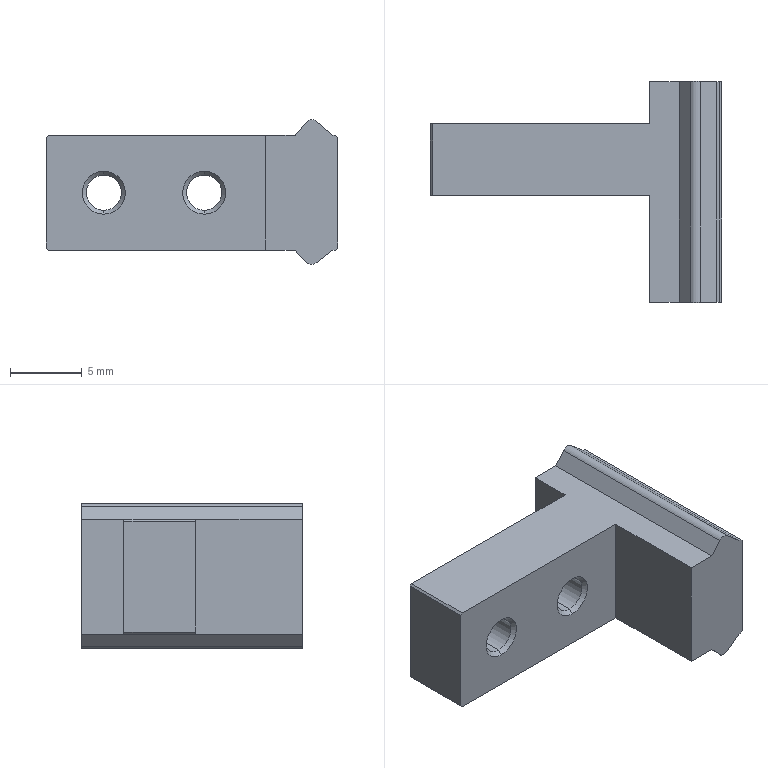Part | SolidWorks | features BaseBody 1 | 1 solid | 35 faces | box 20.3 x 15.4 x 10.1 mm | volume 1229 mm3 | plane 20 | cone 8 | cylinder 7 | commonest cylinder face diameters 2.459 x4 1 x3
STEP:
#1=CARTESIAN_POINT('',(-55.8,12.19,-1.229));
#2=VERTEX_POINT('',#1);
#3=CARTESIAN_POINT('',(-55.8,12.19,1.229));
#4=VERTEX_POINT('',#3);
#5=CARTESIAN_POINT('',(-55.8,12.19,0.));
#6=DIRECTION('',(0.,1.,0.));
#7=DIRECTION('',(0.,0.,1.));
#8=AXIS2_PLACEMENT_3D('',#5,#6,#7);
#9=CIRCLE('',#8,1.229);
#10=EDGE_CURVE('',#2,#4,#9,.T.);
#11=ORIENTED_EDGE('',*,*,#10,.F.);
#12=CARTESIAN_POINT('',(-55.8,12.46,-1.5));
#13=VERTEX_POINT('',#12);
#14=CARTESIAN_POINT('',(-55.8,12.19,-1.229));
#15=DIRECTION('',(0.,0.7071,-0.7071));
#16=VECTOR('',#15,1000.);
#17=LINE('',#14,#16);
#18=EDGE_CURVE('',#2,#13,#17,.T.);
#19=ORIENTED_EDGE('',*,*,#18,.T.);
#20=CARTESIAN_POINT('',(-55.8,12.46,1.5));
#21=VERTEX_POINT('',#20);
#22=CARTESIAN_POINT('',(-55.8,12.46,0.));
#23=DIRECTION('',(0.,1.,0.));
#24=DIRECTION('',(0.,0.,1.));
#25=AXIS2_PLACEMENT_3D('',#22,#23,#24);
#26=CIRCLE('',#25,1.5);
#27=EDGE_CURVE('',#13,#21,#26,.T.);
#28=ORIENTED_EDGE('',*,*,#27,.T.);
#29=CARTESIAN_POINT('',(-55.8,12.19,1.229));
#30=DIRECTION('',(0.,0.7071,0.7071));
#31=VECTOR('',#30,1000.);
#32=LINE('',#29,#31);
#33=EDGE_CURVE('',#4,#21,#32,.T.);
#34=ORIENTED_EDGE('',*,*,#33,.F.);
#35=EDGE_LOOP('',(#11,#19,#28,#34));
#36=FACE_OUTER_BOUND('',#35,.T.);
#37=CARTESIAN_POINT('',(-55.8,12.19,0.));
#38=DIRECTION('',(0.,1.,0.));
#39=DIRECTION('',(0.,0.,1.));
#40=AXIS2_PLACEMENT_3D('',#37,#38,#39);
#41=CONICAL_SURFACE('',#40,1.229,0.7854);
#42=ADVANCED_FACE('',(#36),#41,.F.);
#43=CARTESIAN_POINT('',(-55.8,7.721,-1.229));
#44=VERTEX_POINT('',#43);
#45=CARTESIAN_POINT('',(-55.8,7.721,1.229));
#46=VERTEX_POINT('',#45);
#47=CARTESIAN_POINT('',(-55.8,7.721,0.));
#48=DIRECTION('',(0.,1.,0.));
#49=DIRECTION('',(0.,0.,1.));
#50=AXIS2_PLACEMENT_3D('',#47,#48,#49);
#51=CIRCLE('',#50,1.229);
#52=EDGE_CURVE('',#44,#46,#51,.T.);
#53=ORIENTED_EDGE('',*,*,#52,.F.);
#54=CARTESIAN_POINT('',(-55.8,12.46,-1.229));
#55=DIRECTION('',(0.,1.,0.));
#56=VECTOR('',#55,1000.);
#57=LINE('',#54,#56);
#58=EDGE_CURVE('',#44,#2,#57,.T.);
#59=ORIENTED_EDGE('',*,*,#58,.T.);
#60=ORIENTED_EDGE('',*,*,#10,.T.);
#61=CARTESIAN_POINT('',(-55.8,12.46,1.229));
#62=DIRECTION('',(0.,1.,0.));
#63=VECTOR('',#62,1000.);
#64=LINE('',#61,#63);
#65=EDGE_CURVE('',#46,#4,#64,.T.);
#66=ORIENTED_EDGE('',*,*,#65,.F.);
#67=EDGE_LOOP('',(#53,#59,#60,#66));
#68=FACE_OUTER_BOUND('',#67,.T.);
#69=CARTESIAN_POINT('',(-55.8,12.46,0.));
#70=DIRECTION('',(0.,1.,0.));
#71=DIRECTION('',(0.,0.,1.));
#72=AXIS2_PLACEMENT_3D('',#69,#70,#71);
#73=CYLINDRICAL_SURFACE('',#72,1.229);
#74=ADVANCED_FACE('',(#68),#73,.F.);
#75=ORIENTED_EDGE('',*,*,#52,.T.);
#76=CARTESIAN_POINT('',(-55.8,7.45,1.5));
#77=VERTEX_POINT('',#76);
#78=CARTESIAN_POINT('',(-55.8,7.45,1.5));
#79=DIRECTION('',(0.,-0.7071,0.7071));
#80=VECTOR('',#79,1000.);
#81=LINE('',#78,#80);
#82=EDGE_CURVE('',#46,#77,#81,.T.);
#83=ORIENTED_EDGE('',*,*,#82,.T.);
#84=CARTESIAN_POINT('',(-55.8,7.45,-1.5));
#85=VERTEX_POINT('',#84);
#86=CARTESIAN_POINT('',(-55.8,7.45,0.));
#87=DIRECTION('',(0.,1.,0.));
#88=DIRECTION('',(0.,0.,1.));
#89=AXIS2_PLACEMENT_3D('',#86,#87,#88);
#90=CIRCLE('',#89,1.5);
#91=EDGE_CURVE('',#85,#77,#90,.T.);
#92=ORIENTED_EDGE('',*,*,#91,.F.);
#93=CARTESIAN_POINT('',(-55.8,7.45,-1.5));
#94=DIRECTION('',(0.,-0.7071,-0.7071));
#95=VECTOR('',#94,1000.);
#96=LINE('',#93,#95);
#97=EDGE_CURVE('',#44,#85,#96,.T.);
#98=ORIENTED_EDGE('',*,*,#97,.F.);
#99=EDGE_LOOP('',(#75,#83,#92,#98));
#100=FACE_OUTER_BOUND('',#99,.T.);
#101=CARTESIAN_POINT('',(-55.8,7.45,0.));
#102=DIRECTION('',(0.,-1.,0.));
#103=DIRECTION('',(0.,0.,-1.));
#104=AXIS2_PLACEMENT_3D('',#101,#102,#103);
#105=CONICAL_SURFACE('',#104,1.5,0.7854);
#106=ADVANCED_FACE('',(#100),#105,.F.);
#107=CARTESIAN_POINT('',(-62.8,12.19,-1.229));
#108=VERTEX_POINT('',#107);
#109=CARTESIAN_POINT('',(-62.8,12.19,1.229));
#110=VERTEX_POINT('',#109);
#111=CARTESIAN_POINT('',(-62.8,12.19,0.));
#112=DIRECTION('',(0.,1.,0.));
#113=DIRECTION('',(0.,0.,1.));
#114=AXIS2_PLACEMENT_3D('',#111,#112,#113);
#115=CIRCLE('',#114,1.229);
#116=EDGE_CURVE('',#108,#110,#115,.T.);
#117=ORIENTED_EDGE('',*,*,#116,.F.);
#118=CARTESIAN_POINT('',(-62.8,12.46,-1.5));
#119=VERTEX_POINT('',#118);
#120=CARTESIAN_POINT('',(-62.8,12.19,-1.229));
#121=DIRECTION('',(0.,0.7071,-0.7071));
#122=VECTOR('',#121,1000.);
#123=LINE('',#120,#122);
#124=EDGE_CURVE('',#108,#119,#123,.T.);
#125=ORIENTED_EDGE('',*,*,#124,.T.);
#126=CARTESIAN_POINT('',(-62.8,12.46,1.5));
#127=VERTEX_POINT('',#126);
#128=CARTESIAN_POINT('',(-62.8,12.46,0.));
#129=DIRECTION('',(0.,1.,0.));
#130=DIRECTION('',(0.,0.,1.));
#131=AXIS2_PLACEMENT_3D('',#128,#129,#130);
#132=CIRCLE('',#131,1.5);
#133=EDGE_CURVE('',#119,#127,#132,.T.);
#134=ORIENTED_EDGE('',*,*,#133,.T.);
#135=CARTESIAN_POINT('',(-62.8,12.19,1.229));
#136=DIRECTION('',(0.,0.7071,0.7071));
#137=VECTOR('',#136,1000.);
#138=LINE('',#135,#137);
#139=EDGE_CURVE('',#110,#127,#138,.T.);
#140=ORIENTED_EDGE('',*,*,#139,.F.);
#141=EDGE_LOOP('',(#117,#125,#134,#140));
#142=FACE_OUTER_BOUND('',#141,.T.);
#143=CARTESIAN_POINT('',(-62.8,12.19,0.));
#144=DIRECTION('',(0.,1.,0.));
#145=DIRECTION('',(0.,0.,1.));
#146=AXIS2_PLACEMENT_3D('',#143,#144,#145);
#147=CONICAL_SURFACE('',#146,1.229,0.7854);
#148=ADVANCED_FACE('',(#142),#147,.F.);
#149=CARTESIAN_POINT('',(-62.8,7.721,-1.229));
#150=VERTEX_POINT('',#149);
#151=CARTESIAN_POINT('',(-62.8,7.721,1.229));
#152=VERTEX_POINT('',#151);
#153=CARTESIAN_POINT('',(-62.8,7.721,0.));
#154=DIRECTION('',(0.,1.,0.));
#155=DIRECTION('',(0.,0.,1.));
#156=AXIS2_PLACEMENT_3D('',#153,#154,#155);
#157=CIRCLE('',#156,1.229);
#158=EDGE_CURVE('',#150,#152,#157,.T.);
#159=ORIENTED_EDGE('',*,*,#158,.F.);
#160=CARTESIAN_POINT('',(-62.8,12.46,-1.229));
#161=DIRECTION('',(0.,1.,0.));
#162=VECTOR('',#161,1000.);
#163=LINE('',#160,#162);
#164=EDGE_CURVE('',#150,#108,#163,.T.);
#165=ORIENTED_EDGE('',*,*,#164,.T.);
#166=ORIENTED_EDGE('',*,*,#116,.T.);
#167=CARTESIAN_POINT('',(-62.8,12.46,1.229));
#168=DIRECTION('',(0.,1.,0.));
#169=VECTOR('',#168,1000.);
#170=LINE('',#167,#169);
#171=EDGE_CURVE('',#152,#110,#170,.T.);
#172=ORIENTED_EDGE('',*,*,#171,.F.);
#173=EDGE_LOOP('',(#159,#165,#166,#172));
#174=FACE_OUTER_BOUND('',#173,.T.);
#175=CARTESIAN_POINT('',(-62.8,12.46,0.));
#176=DIRECTION('',(0.,1.,0.));
#177=DIRECTION('',(0.,0.,1.));
#178=AXIS2_PLACEMENT_3D('',#175,#176,#177);
#179=CYLINDRICAL_SURFACE('',#178,1.229);
#180=ADVANCED_FACE('',(#174),#179,.F.);
#181=ORIENTED_EDGE('',*,*,#158,.T.);
#182=CARTESIAN_POINT('',(-62.8,7.45,1.5));
#183=VERTEX_POINT('',#182);
#184=CARTESIAN_POINT('',(-62.8,7.45,1.5));
#185=DIRECTION('',(0.,-0.7071,0.7071));
#186=VECTOR('',#185,1000.);
#187=LINE('',#184,#186);
#188=EDGE_CURVE('',#152,#183,#187,.T.);
#189=ORIENTED_EDGE('',*,*,#188,.T.);
#190=CARTESIAN_POINT('',(-62.8,7.45,-1.5));
#191=VERTEX_POINT('',#190);
#192=CARTESIAN_POINT('',(-62.8,7.45,0.));
#193=DIRECTION('',(0.,1.,0.));
#194=DIRECTION('',(0.,0.,1.));
#195=AXIS2_PLACEMENT_3D('',#192,#193,#194);
#196=CIRCLE('',#195,1.5);
#197=EDGE_CURVE('',#191,#183,#196,.T.);
#198=ORIENTED_EDGE('',*,*,#197,.F.);
#199=CARTESIAN_POINT('',(-62.8,7.45,-1.5));
#200=DIRECTION('',(0.,-0.7071,-0.7071));
#201=VECTOR('',#200,1000.);
#202=LINE('',#199,#201);
#203=EDGE_CURVE('',#150,#191,#202,.T.);
#204=ORIENTED_EDGE('',*,*,#203,.F.);
#205=EDGE_LOOP('',(#181,#189,#198,#204));
#206=FACE_OUTER_BOUND('',#205,.T.);
#207=CARTESIAN_POINT('',(-62.8,7.45,0.));
#208=DIRECTION('',(0.,-1.,0.));
#209=DIRECTION('',(0.,0.,-1.));
#210=AXIS2_PLACEMENT_3D('',#207,#208,#209);
#211=CONICAL_SURFACE('',#210,1.5,0.7854);
#212=ADVANCED_FACE('',(#206),#211,.F.);
#213=CARTESIAN_POINT('',(-48.3,15.41,-5.));
#214=VERTEX_POINT('',#213);
#215=CARTESIAN_POINT('',(-48.663,15.41,-4.843));
#216=VERTEX_POINT('',#215);
#217=CARTESIAN_POINT('',(-48.3,15.41,-4.5));
#218=DIRECTION('',(0.,1.,0.));
#219=DIRECTION('',(0.6065,0.,-0.7951));
#220=AXIS2_PLACEMENT_3D('',#217,#218,#219);
#221=CIRCLE('',#220,0.5);
#222=EDGE_CURVE('',#214,#216,#221,.T.);
#223=ORIENTED_EDGE('',*,*,#222,.F.);
#224=CARTESIAN_POINT('',(-48.3,0.01,-5.));
#225=VERTEX_POINT('',#224);
#226=CARTESIAN_POINT('',(-48.3,15.41,-5.));
#227=DIRECTION('',(0.,-1.,0.));
#228=VECTOR('',#227,1000.);
#229=LINE('',#226,#228);
#230=EDGE_CURVE('',#214,#225,#229,.T.);
#231=ORIENTED_EDGE('',*,*,#230,.T.);
#232=CARTESIAN_POINT('',(-48.663,0.01,-4.843));
#233=VERTEX_POINT('',#232);
#234=CARTESIAN_POINT('',(-48.3,0.01,-4.5));
#235=DIRECTION('',(0.,1.,0.));
#236=DIRECTION('',(0.6065,0.,-0.7951));
#237=AXIS2_PLACEMENT_3D('',#234,#235,#236);
#238=CIRCLE('',#237,0.5);
#239=EDGE_CURVE('',#225,#233,#238,.T.);
#240=ORIENTED_EDGE('',*,*,#239,.T.);
#241=CARTESIAN_POINT('',(-48.663,15.41,-4.843));
#242=DIRECTION('',(0.,-1.,0.));
#243=VECTOR('',#242,1000.);
#244=LINE('',#241,#243);
#245=EDGE_CURVE('',#216,#233,#244,.T.);
#246=ORIENTED_EDGE('',*,*,#245,.F.);
#247=EDGE_LOOP('',(#223,#231,#240,#246));
#248=FACE_OUTER_BOUND('',#247,.T.);
#249=CARTESIAN_POINT('',(-48.3,15.41,-4.5));
#250=DIRECTION('',(0.,-1.,0.));
#251=DIRECTION('',(0.,0.,-1.));
#252=AXIS2_PLACEMENT_3D('',#249,#250,#251);
#253=CYLINDRICAL_SURFACE('',#252,0.5);
#254=ADVANCED_FACE('',(#248),#253,.T.);
#255=CARTESIAN_POINT('',(-51.5,12.46,4.));
#256=VERTEX_POINT('',#255);
#257=CARTESIAN_POINT('',(-51.5,12.46,-4.));
#258=VERTEX_POINT('',#257);
#259=CARTESIAN_POINT('',(-51.5,12.46,4.));
#260=DIRECTION('',(0.,0.,-1.));
#261=VECTOR('',#260,1000.);
#262=LINE('',#259,#261);
#263=EDGE_CURVE('',#256,#258,#262,.T.);
#264=ORIENTED_EDGE('',*,*,#263,.F.);
#265=CARTESIAN_POINT('',(-51.5,15.41,4.));
#266=VERTEX_POINT('',#265);
#267=CARTESIAN_POINT('',(-51.5,15.41,4.));
#268=DIRECTION('',(0.,-1.,0.));
#269=VECTOR('',#268,1000.);
#270=LINE('',#267,#269);
#271=EDGE_CURVE('',#266,#256,#270,.T.);
#272=ORIENTED_EDGE('',*,*,#271,.F.);
#273=CARTESIAN_POINT('',(-51.5,15.41,-4.));
#274=VERTEX_POINT('',#273);
#275=CARTESIAN_POINT('',(-51.5,15.41,-4.));
#276=DIRECTION('',(0.,0.,1.));
#277=VECTOR('',#276,1000.);
#278=LINE('',#275,#277);
#279=EDGE_CURVE('',#274,#266,#278,.T.);
#280=ORIENTED_EDGE('',*,*,#279,.F.);
#281=CARTESIAN_POINT('',(-51.5,15.41,-4.));
#282=DIRECTION('',(0.,-1.,0.));
#283=VECTOR('',#282,1000.);
#284=LINE('',#281,#283);
#285=EDGE_CURVE('',#274,#258,#284,.T.);
#286=ORIENTED_EDGE('',*,*,#285,.T.);
#287=EDGE_LOOP('',(#264,#272,#280,#286));
#288=FACE_OUTER_BOUND('',#287,.T.);
#289=CARTESIAN_POINT('',(-51.5,15.41,-4.));
#290=DIRECTION('',(1.,0.,0.));
#291=DIRECTION('',(0.,0.,-1.));
#292=AXIS2_PLACEMENT_3D('',#289,#290,#291);
#293=PLANE('',#292);
#294=ADVANCED_FACE('',(#288),#293,.F.);
#295=CARTESIAN_POINT('',(-51.5,7.45,4.));
#296=VERTEX_POINT('',#295);
#297=CARTESIAN_POINT('',(-51.5,0.01,4.));
#298=VERTEX_POINT('',#297);
#299=CARTESIAN_POINT('',(-51.5,7.45,4.));
#300=DIRECTION('',(0.,-1.,0.));
#301=VECTOR('',#300,1000.);
#302=LINE('',#299,#301);
#303=EDGE_CURVE('',#296,#298,#302,.T.);
#304=ORIENTED_EDGE('',*,*,#303,.F.);
#305=CARTESIAN_POINT('',(-51.5,7.45,-4.));
#306=VERTEX_POINT('',#305);
#307=CARTESIAN_POINT('',(-51.5,7.45,4.));
#308=DIRECTION('',(0.,0.,-1.));
#309=VECTOR('',#308,1000.);
#310=LINE('',#307,#309);
#311=EDGE_CURVE('',#296,#306,#310,.T.);
#312=ORIENTED_EDGE('',*,*,#311,.T.);
#313=CARTESIAN_POINT('',(-51.5,0.01,-4.));
#314=VERTEX_POINT('',#313);
#315=CARTESIAN_POINT('',(-51.5,7.45,-4.));
#316=DIRECTION('',(0.,-1.,0.));
#317=VECTOR('',#316,1000.);
#318=LINE('',#315,#317);
#319=EDGE_CURVE('',#306,#314,#318,.T.);
#320=ORIENTED_EDGE('',*,*,#319,.T.);
#321=CARTESIAN_POINT('',(-51.5,0.01,-4.));
#322=DIRECTION('',(0.,0.,1.));
#323=VECTOR('',#322,1000.);
#324=LINE('',#321,#323);
#325=EDGE_CURVE('',#314,#298,#324,.T.);
#326=ORIENTED_EDGE('',*,*,#325,.T.);
#327=EDGE_LOOP('',(#304,#312,#320,#326));
#328=FACE_OUTER_BOUND('',#327,.T.);
#329=CARTESIAN_POINT('',(-51.5,15.41,-4.));
#330=DIRECTION('',(1.,0.,0.));
#331=DIRECTION('',(0.,0.,-1.));
#332=AXIS2_PLACEMENT_3D('',#329,#330,#331);
#333=PLANE('',#332);
#334=ADVANCED_FACE('',(#328),#333,.F.);
#335=CARTESIAN_POINT('',(-49.46,0.01,4.));
#336=VERTEX_POINT('',#335);
#337=CARTESIAN_POINT('',(-51.5,0.01,4.));
#338=DIRECTION('',(1.,0.,0.));
#339=VECTOR('',#338,1000.);
#340=LINE('',#337,#339);
#341=EDGE_CURVE('',#298,#336,#340,.T.);
#342=ORIENTED_EDGE('',*,*,#341,.T.);
#343=CARTESIAN_POINT('',(-49.46,15.41,4.));
#344=VERTEX_POINT('',#343);
#345=CARTESIAN_POINT('',(-49.46,15.41,4.));
#346=DIRECTION('',(0.,-1.,0.));
#347=VECTOR('',#346,1000.);
#348=LINE('',#345,#347);
#349=EDGE_CURVE('',#344,#336,#348,.T.);
#350=ORIENTED_EDGE('',*,*,#349,.F.);
#351=CARTESIAN_POINT('',(-51.5,15.41,4.));
#352=DIRECTION('',(1.,0.,0.));
#353=VECTOR('',#352,1000.);
#354=LINE('',#351,#353);
#355=EDGE_CURVE('',#266,#344,#354,.T.);
#356=ORIENTED_EDGE('',*,*,#355,.F.);
#357=ORIENTED_EDGE('',*,*,#271,.T.);
#358=CARTESIAN_POINT('',(-66.659,12.46,4.));
#359=VERTEX_POINT('',#358);
#360=CARTESIAN_POINT('',(-66.659,12.46,4.));
#361=DIRECTION('',(1.,0.,0.));
#362=VECTOR('',#361,1000.);
#363=LINE('',#360,#362);
#364=EDGE_CURVE('',#359,#256,#363,.T.);
#365=ORIENTED_EDGE('',*,*,#364,.F.);
#366=CARTESIAN_POINT('',(-66.659,7.45,4.));
#367=VERTEX_POINT('',#366);
#368=CARTESIAN_POINT('',(-66.659,12.46,4.));
#369=DIRECTION('',(0.,-1.,0.));
#370=VECTOR('',#369,1000.);
#371=LINE('',#368,#370);
#372=EDGE_CURVE('',#359,#367,#371,.T.);
#373=ORIENTED_EDGE('',*,*,#372,.T.);
#374=CARTESIAN_POINT('',(-66.659,7.45,4.));
#375=DIRECTION('',(1.,0.,0.));
#376=VECTOR('',#375,1000.);
#377=LINE('',#374,#376);
#378=EDGE_CURVE('',#367,#296,#377,.T.);
#379=ORIENTED_EDGE('',*,*,#378,.T.);
#380=ORIENTED_EDGE('',*,*,#303,.T.);
#381=EDGE_LOOP('',(#342,#350,#356,#357,#365,#373,#379,#380));
#382=FACE_OUTER_BOUND('',#381,.T.);
#383=CARTESIAN_POINT('',(-51.5,15.41,4.));
#384=DIRECTION('',(0.,0.,-1.));
#385=DIRECTION('',(-1.,0.,0.));
#386=AXIS2_PLACEMENT_3D('',#383,#384,#385);
#387=PLANE('',#386);
#388=ADVANCED_FACE('',(#382),#387,.F.);
#389=CARTESIAN_POINT('',(-48.682,0.01,4.922));
#390=VERTEX_POINT('',#389);
#391=CARTESIAN_POINT('',(-49.46,0.01,4.));
#392=DIRECTION('',(0.6447,0.,0.7645));
#393=VECTOR('',#392,1000.);
#394=LINE('',#391,#393);
#395=EDGE_CURVE('',#336,#390,#394,.T.);
#396=ORIENTED_EDGE('',*,*,#395,.T.);
#397=CARTESIAN_POINT('',(-48.682,15.41,4.922));
#398=VERTEX_POINT('',#397);
#399=CARTESIAN_POINT('',(-48.682,15.41,4.922));
#400=DIRECTION('',(0.,-1.,0.));
#401=VECTOR('',#400,1000.);
#402=LINE('',#399,#401);
#403=EDGE_CURVE('',#398,#390,#402,.T.);
#404=ORIENTED_EDGE('',*,*,#403,.F.);
#405=CARTESIAN_POINT('',(-49.46,15.41,4.));
#406=DIRECTION('',(0.6447,0.,0.7645));
#407=VECTOR('',#406,1000.);
#408=LINE('',#405,#407);
#409=EDGE_CURVE('',#344,#398,#408,.T.);
#410=ORIENTED_EDGE('',*,*,#409,.F.);
#411=ORIENTED_EDGE('',*,*,#349,.T.);
#412=EDGE_LOOP('',(#396,#404,#410,#411));
#413=FACE_OUTER_BOUND('',#412,.T.);
#414=CARTESIAN_POINT('',(-49.46,15.41,4.));
#415=DIRECTION('',(0.7645,0.,-0.6447));
#416=DIRECTION('',(-0.6447,0.,-0.7645));
#417=AXIS2_PLACEMENT_3D('',#414,#415,#416);
#418=PLANE('',#417);
#419=ADVANCED_FACE('',(#413),#418,.F.);
#420=CARTESIAN_POINT('',(-47.977,0.01,4.981));
#421=VERTEX_POINT('',#420);
#422=CARTESIAN_POINT('',(-48.3,0.01,4.6));
#423=DIRECTION('',(0.,1.,0.));
#424=DIRECTION('',(-0.7645,0.,0.6447));
#425=AXIS2_PLACEMENT_3D('',#422,#423,#424);
#426=CIRCLE('',#425,0.5);
#427=EDGE_CURVE('',#390,#421,#426,.T.);
#428=ORIENTED_EDGE('',*,*,#427,.T.);
#429=CARTESIAN_POINT('',(-47.977,15.41,4.981));
#430=VERTEX_POINT('',#429);
#431=CARTESIAN_POINT('',(-47.977,15.41,4.981));
#432=DIRECTION('',(0.,-1.,0.));
#433=VECTOR('',#432,1000.);
#434=LINE('',#431,#433);
#435=EDGE_CURVE('',#430,#421,#434,.T.);
#436=ORIENTED_EDGE('',*,*,#435,.F.);
#437=CARTESIAN_POINT('',(-48.3,15.41,4.6));
#438=DIRECTION('',(0.,1.,0.));
#439=DIRECTION('',(-0.7645,0.,0.6447));
#440=AXIS2_PLACEMENT_3D('',#437,#438,#439);
#441=CIRCLE('',#440,0.5);
#442=EDGE_CURVE('',#398,#430,#441,.T.);
#443=ORIENTED_EDGE('',*,*,#442,.F.);
#444=ORIENTED_EDGE('',*,*,#403,.T.);
#445=EDGE_LOOP('',(#428,#436,#443,#444));
#446=FACE_OUTER_BOUND('',#445,.T.);
#447=CARTESIAN_POINT('',(-48.3,15.41,4.6));
#448=DIRECTION('',(0.,-1.,0.));
#449=DIRECTION('',(0.,0.,-1.));
#450=AXIS2_PLACEMENT_3D('',#447,#448,#449);
#451=CYLINDRICAL_SURFACE('',#450,0.5);
#452=ADVANCED_FACE('',(#446),#451,.T.);
#453=CARTESIAN_POINT('',(-46.82,0.01,4.));
#454=VERTEX_POINT('',#453);
#455=CARTESIAN_POINT('',(-47.977,0.01,4.981));
#456=DIRECTION('',(0.7625,0.,-0.647));
#457=VECTOR('',#456,1000.);
#458=LINE('',#455,#457);
#459=EDGE_CURVE('',#421,#454,#458,.T.);
#460=ORIENTED_EDGE('',*,*,#459,.T.);
#461=CARTESIAN_POINT('',(-46.82,15.41,4.));
#462=VERTEX_POINT('',#461);
#463=CARTESIAN_POINT('',(-46.82,15.41,4.));
#464=DIRECTION('',(0.,-1.,0.));
#465=VECTOR('',#464,1000.);
#466=LINE('',#463,#465);
#467=EDGE_CURVE('',#462,#454,#466,.T.);
#468=ORIENTED_EDGE('',*,*,#467,.F.);
#469=CARTESIAN_POINT('',(-47.977,15.41,4.981));
#470=DIRECTION('',(0.7625,0.,-0.647));
#471=VECTOR('',#470,1000.);
#472=LINE('',#469,#471);
#473=EDGE_CURVE('',#430,#462,#472,.T.);
#474=ORIENTED_EDGE('',*,*,#473,.F.);
#475=ORIENTED_EDGE('',*,*,#435,.T.);
#476=EDGE_LOOP('',(#460,#468,#474,#475));
#477=FACE_OUTER_BOUND('',#476,.T.);
#478=CARTESIAN_POINT('',(-47.977,15.41,4.981));
#479=DIRECTION('',(-0.647,0.,-0.7625));
#480=DIRECTION('',(-0.7625,0.,0.647));
#481=AXIS2_PLACEMENT_3D('',#478,#479,#480);
#482=PLANE('',#481);
#483=ADVANCED_FACE('',(#477),#482,.F.);
#484=CARTESIAN_POINT('',(-46.641,0.01,4.));
#485=VERTEX_POINT('',#484);
#486=CARTESIAN_POINT('',(-46.82,0.01,4.));
#487=DIRECTION('',(1.,0.,0.));
#488=VECTOR('',#487,1000.);
#489=LINE('',#486,#488);
#490=EDGE_CURVE('',#454,#485,#489,.T.);
#491=ORIENTED_EDGE('',*,*,#490,.T.);
#492=CARTESIAN_POINT('',(-46.641,15.41,4.));
#493=VERTEX_POINT('',#492);
#494=CARTESIAN_POINT('',(-46.641,15.41,4.));
#495=DIRECTION('',(0.,-1.,0.));
#496=VECTOR('',#495,1000.);
#497=LINE('',#494,#496);
#498=EDGE_CURVE('',#493,#485,#497,.T.);
#499=ORIENTED_EDGE('',*,*,#498,.F.);
#500=CARTESIAN_POINT('',(-46.82,15.41,4.));
#501=DIRECTION('',(1.,0.,0.));
#502=VECTOR('',#501,1000.);
#503=LINE('',#500,#502);
#504=EDGE_CURVE('',#462,#493,#503,.T.);
#505=ORIENTED_EDGE('',*,*,#504,.F.);
#506=ORIENTED_EDGE('',*,*,#467,.T.);
#507=EDGE_LOOP('',(#491,#499,#505,#506));
#508=FACE_OUTER_BOUND('',#507,.T.);
#509=CARTESIAN_POINT('',(-46.82,15.41,4.));
#510=DIRECTION('',(0.,0.,-1.));
#511=DIRECTION('',(-1.,0.,0.));
#512=AXIS2_PLACEMENT_3D('',#509,#510,#511);
#513=PLANE('',#512);
#514=ADVANCED_FACE('',(#508),#513,.F.);
#515=CARTESIAN_POINT('',(-46.5,0.01,3.859));
#516=VERTEX_POINT('',#515);
#517=CARTESIAN_POINT('',(-46.641,0.01,4.));
#518=DIRECTION('',(0.7071,0.,-0.7071));
#519=VECTOR('',#518,1000.);
#520=LINE('',#517,#519);
#521=EDGE_CURVE('',#485,#516,#520,.T.);
#522=ORIENTED_EDGE('',*,*,#521,.T.);
#523=CARTESIAN_POINT('',(-46.5,15.41,3.859));
#524=VERTEX_POINT('',#523);
#525=CARTESIAN_POINT('',(-46.5,15.41,3.859));
#526=DIRECTION('',(0.,-1.,0.));
#527=VECTOR('',#526,1000.);
#528=LINE('',#525,#527);
#529=EDGE_CURVE('',#524,#516,#528,.T.);
#530=ORIENTED_EDGE('',*,*,#529,.F.);
#531=CARTESIAN_POINT('',(-46.641,15.41,4.));
#532=DIRECTION('',(0.7071,0.,-0.7071));
#533=VECTOR('',#532,1000.);
#534=LINE('',#531,#533);
#535=EDGE_CURVE('',#493,#524,#534,.T.);
#536=ORIENTED_EDGE('',*,*,#535,.F.);
#537=ORIENTED_EDGE('',*,*,#498,.T.);
#538=EDGE_LOOP('',(#522,#530,#536,#537));
#539=FACE_OUTER_BOUND('',#538,.T.);
#540=CARTESIAN_POINT('',(-46.641,15.41,4.));
#541=DIRECTION('',(-0.7071,0.,-0.7071));
#542=DIRECTION('',(-0.7071,0.,0.7071));
#543=AXIS2_PLACEMENT_3D('',#540,#541,#542);
#544=PLANE('',#543);
#545=ADVANCED_FACE('',(#539),#544,.F.);
#546=CARTESIAN_POINT('',(-46.5,0.01,-3.859));
#547=VERTEX_POINT('',#546);
#548=CARTESIAN_POINT('',(-46.5,0.01,3.859));
#549=DIRECTION('',(0.,0.,-1.));
#550=VECTOR('',#549,1000.);
#551=LINE('',#548,#550);
#552=EDGE_CURVE('',#516,#547,#551,.T.);
#553=ORIENTED_EDGE('',*,*,#552,.T.);
#554=CARTESIAN_POINT('',(-46.5,15.41,-3.859));
#555=VERTEX_POINT('',#554);
#556=CARTESIAN_POINT('',(-46.5,15.41,-3.859));
#557=DIRECTION('',(0.,-1.,0.));
#558=VECTOR('',#557,1000.);
#559=LINE('',#556,#558);
#560=EDGE_CURVE('',#555,#547,#559,.T.);
#561=ORIENTED_EDGE('',*,*,#560,.F.);
#562=CARTESIAN_POINT('',(-46.5,15.41,3.859));
#563=DIRECTION('',(0.,0.,-1.));
#564=VECTOR('',#563,1000.);
#565=LINE('',#562,#564);
#566=EDGE_CURVE('',#524,#555,#565,.T.);
#567=ORIENTED_EDGE('',*,*,#566,.F.);
#568=ORIENTED_EDGE('',*,*,#529,.T.);
#569=EDGE_LOOP('',(#553,#561,#567,#568));
#570=FACE_OUTER_BOUND('',#569,.T.);
#571=CARTESIAN_POINT('',(-46.5,15.41,3.859));
#572=DIRECTION('',(-1.,0.,0.));
#573=DIRECTION('',(0.,0.,1.));
#574=AXIS2_PLACEMENT_3D('',#571,#572,#573);
#575=PLANE('',#574);
#576=ADVANCED_FACE('',(#570),#575,.F.);
#577=CARTESIAN_POINT('',(-46.641,0.01,-4.));
#578=VERTEX_POINT('',#577);
#579=CARTESIAN_POINT('',(-46.5,0.01,-3.859));
#580=DIRECTION('',(-0.7071,0.,-0.7071));
#581=VECTOR('',#580,1000.);
#582=LINE('',#579,#581);
#583=EDGE_CURVE('',#547,#578,#582,.T.);
#584=ORIENTED_EDGE('',*,*,#583,.T.);
#585=CARTESIAN_POINT('',(-46.641,15.41,-4.));
#586=VERTEX_POINT('',#585);
#587=CARTESIAN_POINT('',(-46.641,15.41,-4.));
#588=DIRECTION('',(0.,-1.,0.));
#589=VECTOR('',#588,1000.);
#590=LINE('',#587,#589);
#591=EDGE_CURVE('',#586,#578,#590,.T.);
#592=ORIENTED_EDGE('',*,*,#591,.F.);
#593=CARTESIAN_POINT('',(-46.5,15.41,-3.859));
#594=DIRECTION('',(-0.7071,0.,-0.7071));
#595=VECTOR('',#594,1000.);
#596=LINE('',#593,#595);
#597=EDGE_CURVE('',#555,#586,#596,.T.);
#598=ORIENTED_EDGE('',*,*,#597,.F.);
#599=ORIENTED_EDGE('',*,*,#560,.T.);
#600=EDGE_LOOP('',(#584,#592,#598,#599));
#601=FACE_OUTER_BOUND('',#600,.T.);
#602=CARTESIAN_POINT('',(-46.5,15.41,-3.859));
#603=DIRECTION('',(-0.7071,0.,0.7071));
#604=DIRECTION('',(0.7071,0.,0.7071));
#605=AXIS2_PLACEMENT_3D('',#602,#603,#604);
#606=PLANE('',#605);
#607=ADVANCED_FACE('',(#601),#606,.F.);
#608=CARTESIAN_POINT('',(-46.82,0.01,-4.));
#609=VERTEX_POINT('',#608);
#610=CARTESIAN_POINT('',(-46.641,0.01,-4.));
#611=DIRECTION('',(-1.,0.,0.));
#612=VECTOR('',#611,1000.);
#613=LINE('',#610,#612);
#614=EDGE_CURVE('',#578,#609,#613,.T.);
#615=ORIENTED_EDGE('',*,*,#614,.T.);
#616=CARTESIAN_POINT('',(-46.82,15.41,-4.));
#617=VERTEX_POINT('',#616);
#618=CARTESIAN_POINT('',(-46.82,15.41,-4.));
#619=DIRECTION('',(0.,-1.,0.));
#620=VECTOR('',#619,1000.);
#621=LINE('',#618,#620);
#622=EDGE_CURVE('',#617,#609,#621,.T.);
#623=ORIENTED_EDGE('',*,*,#622,.F.);
#624=CARTESIAN_POINT('',(-46.641,15.41,-4.));
#625=DIRECTION('',(-1.,0.,0.));
#626=VECTOR('',#625,1000.);
#627=LINE('',#624,#626);
#628=EDGE_CURVE('',#586,#617,#627,.T.);
#629=ORIENTED_EDGE('',*,*,#628,.F.);
#630=ORIENTED_EDGE('',*,*,#591,.T.);
#631=EDGE_LOOP('',(#615,#623,#629,#630));
#632=FACE_OUTER_BOUND('',#631,.T.);
#633=CARTESIAN_POINT('',(-46.641,15.41,-4.));
#634=DIRECTION('',(0.,0.,1.));
#635=DIRECTION('',(1.,0.,0.));
#636=AXIS2_PLACEMENT_3D('',#633,#634,#635);
#637=PLANE('',#636);
#638=ADVANCED_FACE('',(#632),#637,.F.);
#639=CARTESIAN_POINT('',(-47.997,0.01,-4.898));
#640=VERTEX_POINT('',#639);
#641=CARTESIAN_POINT('',(-46.82,0.01,-4.));
#642=DIRECTION('',(-0.7951,0.,-0.6065));
#643=VECTOR('',#642,1000.);
#644=LINE('',#641,#643);
#645=EDGE_CURVE('',#609,#640,#644,.T.);
#646=ORIENTED_EDGE('',*,*,#645,.T.);
#647=CARTESIAN_POINT('',(-47.997,15.41,-4.898));
#648=VERTEX_POINT('',#647);
#649=CARTESIAN_POINT('',(-47.997,15.41,-4.898));
#650=DIRECTION('',(0.,-1.,0.));
#651=VECTOR('',#650,1000.);
#652=LINE('',#649,#651);
#653=EDGE_CURVE('',#648,#640,#652,.T.);
#654=ORIENTED_EDGE('',*,*,#653,.F.);
#655=CARTESIAN_POINT('',(-46.82,15.41,-4.));
#656=DIRECTION('',(-0.7951,0.,-0.6065));
#657=VECTOR('',#656,1000.);
#658=LINE('',#655,#657);
#659=EDGE_CURVE('',#617,#648,#658,.T.);
#660=ORIENTED_EDGE('',*,*,#659,.F.);
#661=ORIENTED_EDGE('',*,*,#622,.T.);
#662=EDGE_LOOP('',(#646,#654,#660,#661));
#663=FACE_OUTER_BOUND('',#662,.T.);
#664=CARTESIAN_POINT('',(-46.82,15.41,-4.));
#665=DIRECTION('',(-0.6065,0.,0.7951));
#666=DIRECTION('',(0.7951,0.,0.6065));
#667=AXIS2_PLACEMENT_3D('',#664,#665,#666);
#668=PLANE('',#667);
#669=ADVANCED_FACE('',(#663),#668,.F.);
#670=ORIENTED_EDGE('',*,*,#230,.F.);
#671=CARTESIAN_POINT('',(-48.3,15.41,-4.5));
#672=DIRECTION('',(0.,1.,0.));
#673=DIRECTION('',(0.6065,0.,-0.7951));
#674=AXIS2_PLACEMENT_3D('',#671,#672,#673);
#675=CIRCLE('',#674,0.5);
#676=EDGE_CURVE('',#648,#214,#675,.T.);
#677=ORIENTED_EDGE('',*,*,#676,.F.);
#678=ORIENTED_EDGE('',*,*,#653,.T.);
#679=CARTESIAN_POINT('',(-48.3,0.01,-4.5));
#680=DIRECTION('',(0.,1.,0.));
#681=DIRECTION('',(0.6065,0.,-0.7951));
#682=AXIS2_PLACEMENT_3D('',#679,#680,#681);
#683=CIRCLE('',#682,0.5);
#684=EDGE_CURVE('',#640,#225,#683,.T.);
#685=ORIENTED_EDGE('',*,*,#684,.T.);
#686=EDGE_LOOP('',(#670,#677,#678,#685));
#687=FACE_OUTER_BOUND('',#686,.T.);
#688=CARTESIAN_POINT('',(-48.3,15.41,-4.5));
#689=DIRECTION('',(0.,-1.,0.));
#690=DIRECTION('',(0.,0.,-1.));
#691=AXIS2_PLACEMENT_3D('',#688,#689,#690);
#692=CYLINDRICAL_SURFACE('',#691,0.5);
#693=ADVANCED_FACE('',(#687),#692,.T.);
#694=CARTESIAN_POINT('',(-49.46,0.01,-4.));
#695=VERTEX_POINT('',#694);
#696=CARTESIAN_POINT('',(-48.663,0.01,-4.843));
#697=DIRECTION('',(-0.6866,0.,0.727));
#698=VECTOR('',#697,1000.);
#699=LINE('',#696,#698);
#700=EDGE_CURVE('',#233,#695,#699,.T.);
#701=ORIENTED_EDGE('',*,*,#700,.T.);
#702=CARTESIAN_POINT('',(-49.46,15.41,-4.));
#703=VERTEX_POINT('',#702);
#704=CARTESIAN_POINT('',(-49.46,15.41,-4.));
#705=DIRECTION('',(0.,-1.,0.));
#706=VECTOR('',#705,1000.);
#707=LINE('',#704,#706);
#708=EDGE_CURVE('',#703,#695,#707,.T.);
#709=ORIENTED_EDGE('',*,*,#708,.F.);
#710=CARTESIAN_POINT('',(-48.663,15.41,-4.843));
#711=DIRECTION('',(-0.6866,0.,0.727));
#712=VECTOR('',#711,1000.);
#713=LINE('',#710,#712);
#714=EDGE_CURVE('',#216,#703,#713,.T.);
#715=ORIENTED_EDGE('',*,*,#714,.F.);
#716=ORIENTED_EDGE('',*,*,#245,.T.);
#717=EDGE_LOOP('',(#701,#709,#715,#716));
#718=FACE_OUTER_BOUND('',#717,.T.);
#719=CARTESIAN_POINT('',(-48.663,15.41,-4.843));
#720=DIRECTION('',(0.727,0.,0.6866));
#721=DIRECTION('',(0.6866,0.,-0.727));
#722=AXIS2_PLACEMENT_3D('',#719,#720,#721);
#723=PLANE('',#722);
#724=ADVANCED_FACE('',(#718),#723,.F.);
#725=CARTESIAN_POINT('',(-49.46,0.01,-4.));
#726=DIRECTION('',(-1.,0.,0.));
#727=VECTOR('',#726,1000.);
#728=LINE('',#725,#727);
#729=EDGE_CURVE('',#695,#314,#728,.T.);
#730=ORIENTED_EDGE('',*,*,#729,.T.);
#731=ORIENTED_EDGE('',*,*,#319,.F.);
#732=CARTESIAN_POINT('',(-66.659,7.45,-4.));
#733=VERTEX_POINT('',#732);
#734=CARTESIAN_POINT('',(-51.5,7.45,-4.));
#735=DIRECTION('',(-1.,0.,0.));
#736=VECTOR('',#735,1000.);
#737=LINE('',#734,#736);
#738=EDGE_CURVE('',#306,#733,#737,.T.);
#739=ORIENTED_EDGE('',*,*,#738,.T.);
#740=CARTESIAN_POINT('',(-66.659,12.46,-4.));
#741=VERTEX_POINT('',#740);
#742=CARTESIAN_POINT('',(-66.659,12.46,-4.));
#743=DIRECTION('',(0.,-1.,0.));
#744=VECTOR('',#743,1000.);
#745=LINE('',#742,#744);
#746=EDGE_CURVE('',#741,#733,#745,.T.);
#747=ORIENTED_EDGE('',*,*,#746,.F.);
#748=CARTESIAN_POINT('',(-51.5,12.46,-4.));
#749=DIRECTION('',(-1.,0.,0.));
#750=VECTOR('',#749,1000.);
#751=LINE('',#748,#750);
#752=EDGE_CURVE('',#258,#741,#751,.T.);
#753=ORIENTED_EDGE('',*,*,#752,.F.);
#754=ORIENTED_EDGE('',*,*,#285,.F.);
#755=CARTESIAN_POINT('',(-49.46,15.41,-4.));
#756=DIRECTION('',(-1.,0.,0.));
#757=VECTOR('',#756,1000.);
#758=LINE('',#755,#757);
#759=EDGE_CURVE('',#703,#274,#758,.T.);
#760=ORIENTED_EDGE('',*,*,#759,.F.);
#761=ORIENTED_EDGE('',*,*,#708,.T.);
#762=EDGE_LOOP('',(#730,#731,#739,#747,#753,#754,#760,#761));
#763=FACE_OUTER_BOUND('',#762,.T.);
#764=CARTESIAN_POINT('',(-49.46,15.41,-4.));
#765=DIRECTION('',(0.,0.,1.));
#766=DIRECTION('',(1.,0.,0.));
#767=AXIS2_PLACEMENT_3D('',#764,#765,#766);
#768=PLANE('',#767);
#769=ADVANCED_FACE('',(#763),#768,.F.);
#770=ORIENTED_EDGE('',*,*,#279,.T.);
#771=ORIENTED_EDGE('',*,*,#355,.T.);
#772=ORIENTED_EDGE('',*,*,#409,.T.);
#773=ORIENTED_EDGE('',*,*,#442,.T.);
#774=ORIENTED_EDGE('',*,*,#473,.T.);
#775=ORIENTED_EDGE('',*,*,#504,.T.);
#776=ORIENTED_EDGE('',*,*,#535,.T.);
#777=ORIENTED_EDGE('',*,*,#566,.T.);
#778=ORIENTED_EDGE('',*,*,#597,.T.);
#779=ORIENTED_EDGE('',*,*,#628,.T.);
#780=ORIENTED_EDGE('',*,*,#659,.T.);
#781=ORIENTED_EDGE('',*,*,#676,.T.);
#782=ORIENTED_EDGE('',*,*,#222,.T.);
#783=ORIENTED_EDGE('',*,*,#714,.T.);
#784=ORIENTED_EDGE('',*,*,#759,.T.);
#785=EDGE_LOOP('',(#770,#771,#772,#773,#774,#775,#776,#777,#778,#779,#780,#781,#782,#783,#784));
#786=FACE_OUTER_BOUND('',#785,.T.);
#787=CARTESIAN_POINT('',(-48.3,15.41,4.6));
#788=DIRECTION('',(0.,1.,0.));
#789=DIRECTION('',(0.,0.,1.));
#790=AXIS2_PLACEMENT_3D('',#787,#788,#789);
#791=PLANE('',#790);
#792=ADVANCED_FACE('',(#786),#791,.T.);
#793=ORIENTED_EDGE('',*,*,#325,.F.);
#794=ORIENTED_EDGE('',*,*,#729,.F.);
#795=ORIENTED_EDGE('',*,*,#700,.F.);
#796=ORIENTED_EDGE('',*,*,#239,.F.);
#797=ORIENTED_EDGE('',*,*,#684,.F.);
#798=ORIENTED_EDGE('',*,*,#645,.F.);
#799=ORIENTED_EDGE('',*,*,#614,.F.);
#800=ORIENTED_EDGE('',*,*,#583,.F.);
#801=ORIENTED_EDGE('',*,*,#552,.F.);
#802=ORIENTED_EDGE('',*,*,#521,.F.);
#803=ORIENTED_EDGE('',*,*,#490,.F.);
#804=ORIENTED_EDGE('',*,*,#459,.F.);
#805=ORIENTED_EDGE('',*,*,#427,.F.);
#806=ORIENTED_EDGE('',*,*,#395,.F.);
#807=ORIENTED_EDGE('',*,*,#341,.F.);
#808=EDGE_LOOP('',(#793,#794,#795,#796,#797,#798,#799,#800,#801,#802,#803,#804,#805,#806,#807));
#809=FACE_OUTER_BOUND('',#808,.T.);
#810=CARTESIAN_POINT('',(-48.3,0.01,4.6));
#811=DIRECTION('',(0.,1.,0.));
#812=DIRECTION('',(0.,0.,1.));
#813=AXIS2_PLACEMENT_3D('',#810,#811,#812);
#814=PLANE('',#813);
#815=ADVANCED_FACE('',(#809),#814,.F.);
#816=CARTESIAN_POINT('',(-66.8,7.45,-3.859));
#817=VERTEX_POINT('',#816);
#818=CARTESIAN_POINT('',(-66.659,7.45,-4.));
#819=DIRECTION('',(-0.7071,0.,0.7071));
#820=VECTOR('',#819,1000.);
#821=LINE('',#818,#820);
#822=EDGE_CURVE('',#733,#817,#821,.T.);
#823=ORIENTED_EDGE('',*,*,#822,.T.);
#824=CARTESIAN_POINT('',(-66.8,12.46,-3.859));
#825=VERTEX_POINT('',#824);
#826=CARTESIAN_POINT('',(-66.8,12.46,-3.859));
#827=DIRECTION('',(0.,-1.,0.));
#828=VECTOR('',#827,1000.);
#829=LINE('',#826,#828);
#830=EDGE_CURVE('',#825,#817,#829,.T.);
#831=ORIENTED_EDGE('',*,*,#830,.F.);
#832=CARTESIAN_POINT('',(-66.659,12.46,-4.));
#833=DIRECTION('',(-0.7071,0.,0.7071));
#834=VECTOR('',#833,1000.);
#835=LINE('',#832,#834);
#836=EDGE_CURVE('',#741,#825,#835,.T.);
#837=ORIENTED_EDGE('',*,*,#836,.F.);
#838=ORIENTED_EDGE('',*,*,#746,.T.);
#839=EDGE_LOOP('',(#823,#831,#837,#838));
#840=FACE_OUTER_BOUND('',#839,.T.);
#841=CARTESIAN_POINT('',(-66.659,12.46,-4.));
#842=DIRECTION('',(0.7071,0.,0.7071));
#843=DIRECTION('',(0.7071,0.,-0.7071));
#844=AXIS2_PLACEMENT_3D('',#841,#842,#843);
#845=PLANE('',#844);
#846=ADVANCED_FACE('',(#840),#845,.F.);
#847=CARTESIAN_POINT('',(-66.8,7.45,3.859));
#848=VERTEX_POINT('',#847);
#849=CARTESIAN_POINT('',(-66.8,7.45,-3.859));
#850=DIRECTION('',(0.,0.,1.));
#851=VECTOR('',#850,1000.);
#852=LINE('',#849,#851);
#853=EDGE_CURVE('',#817,#848,#852,.T.);
#854=ORIENTED_EDGE('',*,*,#853,.T.);
#855=CARTESIAN_POINT('',(-66.8,12.46,3.859));
#856=VERTEX_POINT('',#855);
#857=CARTESIAN_POINT('',(-66.8,12.46,3.859));
#858=DIRECTION('',(0.,-1.,0.));
#859=VECTOR('',#858,1000.);
#860=LINE('',#857,#859);
#861=EDGE_CURVE('',#856,#848,#860,.T.);
#862=ORIENTED_EDGE('',*,*,#861,.F.);
#863=CARTESIAN_POINT('',(-66.8,12.46,-3.859));
#864=DIRECTION('',(0.,0.,1.));
#865=VECTOR('',#864,1000.);
#866=LINE('',#863,#865);
#867=EDGE_CURVE('',#825,#856,#866,.T.);
#868=ORIENTED_EDGE('',*,*,#867,.F.);
#869=ORIENTED_EDGE('',*,*,#830,.T.);
#870=EDGE_LOOP('',(#854,#862,#868,#869));
#871=FACE_OUTER_BOUND('',#870,.T.);
#872=CARTESIAN_POINT('',(-66.8,12.46,-3.859));
#873=DIRECTION('',(1.,0.,0.));
#874=DIRECTION('',(0.,0.,-1.));
#875=AXIS2_PLACEMENT_3D('',#872,#873,#874);
#876=PLANE('',#875);
#877=ADVANCED_FACE('',(#871),#876,.F.);
#878=CARTESIAN_POINT('',(-66.8,7.45,3.859));
#879=DIRECTION('',(0.7071,0.,0.7071));
#880=VECTOR('',#879,1000.);
#881=LINE('',#878,#880);
#882=EDGE_CURVE('',#848,#367,#881,.T.);
#883=ORIENTED_EDGE('',*,*,#882,.T.);
#884=ORIENTED_EDGE('',*,*,#372,.F.);
#885=CARTESIAN_POINT('',(-66.8,12.46,3.859));
#886=DIRECTION('',(0.7071,0.,0.7071));
#887=VECTOR('',#886,1000.);
#888=LINE('',#885,#887);
#889=EDGE_CURVE('',#856,#359,#888,.T.);
#890=ORIENTED_EDGE('',*,*,#889,.F.);
#891=ORIENTED_EDGE('',*,*,#861,.T.);
#892=EDGE_LOOP('',(#883,#884,#890,#891));
#893=FACE_OUTER_BOUND('',#892,.T.);
#894=CARTESIAN_POINT('',(-66.8,12.46,3.859));
#895=DIRECTION('',(0.7071,0.,-0.7071));
#896=DIRECTION('',(-0.7071,0.,-0.7071));
#897=AXIS2_PLACEMENT_3D('',#894,#895,#896);
#898=PLANE('',#897);
#899=ADVANCED_FACE('',(#893),#898,.F.);
#900=CARTESIAN_POINT('',(-55.8,12.46,0.));
#901=DIRECTION('',(0.,1.,0.));
#902=DIRECTION('',(0.,0.,1.));
#903=AXIS2_PLACEMENT_3D('',#900,#901,#902);
#904=CIRCLE('',#903,1.5);
#905=EDGE_CURVE('',#21,#13,#904,.T.);
#906=ORIENTED_EDGE('',*,*,#905,.F.);
#907=ORIENTED_EDGE('',*,*,#27,.F.);
#908=EDGE_LOOP('',(#906,#907));
#909=FACE_BOUND('',#908,.T.);
#910=CARTESIAN_POINT('',(-62.8,12.46,0.));
#911=DIRECTION('',(0.,1.,0.));
#912=DIRECTION('',(0.,0.,1.));
#913=AXIS2_PLACEMENT_3D('',#910,#911,#912);
#914=CIRCLE('',#913,1.5);
#915=EDGE_CURVE('',#127,#119,#914,.T.);
#916=ORIENTED_EDGE('',*,*,#915,.F.);
#917=ORIENTED_EDGE('',*,*,#133,.F.);
#918=EDGE_LOOP('',(#916,#917));
#919=FACE_BOUND('',#918,.T.);
#920=ORIENTED_EDGE('',*,*,#836,.T.);
#921=ORIENTED_EDGE('',*,*,#867,.T.);
#922=ORIENTED_EDGE('',*,*,#889,.T.);
#923=ORIENTED_EDGE('',*,*,#364,.T.);
#924=ORIENTED_EDGE('',*,*,#263,.T.);
#925=ORIENTED_EDGE('',*,*,#752,.T.);
#926=EDGE_LOOP('',(#920,#921,#922,#923,#924,#925));
#927=FACE_OUTER_BOUND('',#926,.T.);
#928=CARTESIAN_POINT('',(0.,12.46,0.));
#929=DIRECTION('',(0.,1.,0.));
#930=DIRECTION('',(0.,0.,1.));
#931=AXIS2_PLACEMENT_3D('',#928,#929,#930);
#932=PLANE('',#931);
#933=ADVANCED_FACE('',(#909,#919,#927),#932,.T.);
#934=ORIENTED_EDGE('',*,*,#91,.T.);
#935=CARTESIAN_POINT('',(-55.8,7.45,0.));
#936=DIRECTION('',(0.,1.,0.));
#937=DIRECTION('',(0.,0.,1.));
#938=AXIS2_PLACEMENT_3D('',#935,#936,#937);
#939=CIRCLE('',#938,1.5);
#940=EDGE_CURVE('',#77,#85,#939,.T.);
#941=ORIENTED_EDGE('',*,*,#940,.T.);
#942=EDGE_LOOP('',(#934,#941));
#943=FACE_BOUND('',#942,.T.);
#944=ORIENTED_EDGE('',*,*,#197,.T.);
#945=CARTESIAN_POINT('',(-62.8,7.45,0.));
#946=DIRECTION('',(0.,1.,0.));
#947=DIRECTION('',(0.,0.,1.));
#948=AXIS2_PLACEMENT_3D('',#945,#946,#947);
#949=CIRCLE('',#948,1.5);
#950=EDGE_CURVE('',#183,#191,#949,.T.);
#951=ORIENTED_EDGE('',*,*,#950,.T.);
#952=EDGE_LOOP('',(#944,#951));
#953=FACE_BOUND('',#952,.T.);
#954=ORIENTED_EDGE('',*,*,#822,.F.);
#955=ORIENTED_EDGE('',*,*,#738,.F.);
#956=ORIENTED_EDGE('',*,*,#311,.F.);
#957=ORIENTED_EDGE('',*,*,#378,.F.);
#958=ORIENTED_EDGE('',*,*,#882,.F.);
#959=ORIENTED_EDGE('',*,*,#853,.F.);
#960=EDGE_LOOP('',(#954,#955,#956,#957,#958,#959));
#961=FACE_OUTER_BOUND('',#960,.T.);
#962=CARTESIAN_POINT('',(0.,7.45,0.));
#963=DIRECTION('',(0.,1.,0.));
#964=DIRECTION('',(0.,0.,1.));
#965=AXIS2_PLACEMENT_3D('',#962,#963,#964);
#966=PLANE('',#965);
#967=ADVANCED_FACE('',(#943,#953,#961),#966,.F.);
#968=ORIENTED_EDGE('',*,*,#188,.F.);
#969=CARTESIAN_POINT('',(-62.8,7.721,0.));
#970=DIRECTION('',(0.,1.,0.));
#971=DIRECTION('',(0.,0.,1.));
#972=AXIS2_PLACEMENT_3D('',#969,#970,#971);
#973=CIRCLE('',#972,1.229);
#974=EDGE_CURVE('',#152,#150,#973,.T.);
#975=ORIENTED_EDGE('',*,*,#974,.T.);
#976=ORIENTED_EDGE('',*,*,#203,.T.);
#977=ORIENTED_EDGE('',*,*,#950,.F.);
#978=EDGE_LOOP('',(#968,#975,#976,#977));
#979=FACE_OUTER_BOUND('',#978,.T.);
#980=CARTESIAN_POINT('',(-62.8,7.45,0.));
#981=DIRECTION('',(0.,-1.,0.));
#982=DIRECTION('',(0.,0.,-1.));
#983=AXIS2_PLACEMENT_3D('',#980,#981,#982);
#984=CONICAL_SURFACE('',#983,1.5,0.7854);
#985=ADVANCED_FACE('',(#979),#984,.F.);
#986=ORIENTED_EDGE('',*,*,#164,.F.);
#987=ORIENTED_EDGE('',*,*,#974,.F.);
#988=ORIENTED_EDGE('',*,*,#171,.T.);
#989=CARTESIAN_POINT('',(-62.8,12.19,0.));
#990=DIRECTION('',(0.,1.,0.));
#991=DIRECTION('',(0.,0.,1.));
#992=AXIS2_PLACEMENT_3D('',#989,#990,#991);
#993=CIRCLE('',#992,1.229);
#994=EDGE_CURVE('',#110,#108,#993,.T.);
#995=ORIENTED_EDGE('',*,*,#994,.T.);
#996=EDGE_LOOP('',(#986,#987,#988,#995));
#997=FACE_OUTER_BOUND('',#996,.T.);
#998=CARTESIAN_POINT('',(-62.8,12.46,0.));
#999=DIRECTION('',(0.,1.,0.));
#1000=DIRECTION('',(0.,0.,1.));
#1001=AXIS2_PLACEMENT_3D('',#998,#999,#1000);
#1002=CYLINDRICAL_SURFACE('',#1001,1.229);
#1003=ADVANCED_FACE('',(#997),#1002,.F.);
#1004=ORIENTED_EDGE('',*,*,#124,.F.);
#1005=ORIENTED_EDGE('',*,*,#994,.F.);
#1006=ORIENTED_EDGE('',*,*,#139,.T.);
#1007=ORIENTED_EDGE('',*,*,#915,.T.);
#1008=EDGE_LOOP('',(#1004,#1005,#1006,#1007));
#1009=FACE_OUTER_BOUND('',#1008,.T.);
#1010=CARTESIAN_POINT('',(-62.8,12.19,0.));
#1011=DIRECTION('',(0.,1.,0.));
#1012=DIRECTION('',(0.,0.,1.));
#1013=AXIS2_PLACEMENT_3D('',#1010,#1011,#1012);
#1014=CONICAL_SURFACE('',#1013,1.229,0.7854);
#1015=ADVANCED_FACE('',(#1009),#1014,.F.);
#1016=ORIENTED_EDGE('',*,*,#82,.F.);
#1017=CARTESIAN_POINT('',(-55.8,7.721,0.));
#1018=DIRECTION('',(0.,1.,0.));
#1019=DIRECTION('',(0.,0.,1.));
#1020=AXIS2_PLACEMENT_3D('',#1017,#1018,#1019);
#1021=CIRCLE('',#1020,1.229);
#1022=EDGE_CURVE('',#46,#44,#1021,.T.);
#1023=ORIENTED_EDGE('',*,*,#1022,.T.);
#1024=ORIENTED_EDGE('',*,*,#97,.T.);
#1025=ORIENTED_EDGE('',*,*,#940,.F.);
#1026=EDGE_LOOP('',(#1016,#1023,#1024,#1025));
#1027=FACE_OUTER_BOUND('',#1026,.T.);
#1028=CARTESIAN_POINT('',(-55.8,7.45,0.));
#1029=DIRECTION('',(0.,-1.,0.));
#1030=DIRECTION('',(0.,0.,-1.));
#1031=AXIS2_PLACEMENT_3D('',#1028,#1029,#1030);
#1032=CONICAL_SURFACE('',#1031,1.5,0.7854);
#1033=ADVANCED_FACE('',(#1027),#1032,.F.);
#1034=ORIENTED_EDGE('',*,*,#58,.F.);
#1035=ORIENTED_EDGE('',*,*,#1022,.F.);
#1036=ORIENTED_EDGE('',*,*,#65,.T.);
#1037=CARTESIAN_POINT('',(-55.8,12.19,0.));
#1038=DIRECTION('',(0.,1.,0.));
#1039=DIRECTION('',(0.,0.,1.));
#1040=AXIS2_PLACEMENT_3D('',#1037,#1038,#1039);
#1041=CIRCLE('',#1040,1.229);
#1042=EDGE_CURVE('',#4,#2,#1041,.T.);
#1043=ORIENTED_EDGE('',*,*,#1042,.T.);
#1044=EDGE_LOOP('',(#1034,#1035,#1036,#1043));
#1045=FACE_OUTER_BOUND('',#1044,.T.);
#1046=CARTESIAN_POINT('',(-55.8,12.46,0.));
#1047=DIRECTION('',(0.,1.,0.));
#1048=DIRECTION('',(0.,0.,1.));
#1049=AXIS2_PLACEMENT_3D('',#1046,#1047,#1048);
#1050=CYLINDRICAL_SURFACE('',#1049,1.229);
#1051=ADVANCED_FACE('',(#1045),#1050,.F.);
#1052=ORIENTED_EDGE('',*,*,#18,.F.);
#1053=ORIENTED_EDGE('',*,*,#1042,.F.);
#1054=ORIENTED_EDGE('',*,*,#33,.T.);
#1055=ORIENTED_EDGE('',*,*,#905,.T.);
#1056=EDGE_LOOP('',(#1052,#1053,#1054,#1055));
#1057=FACE_OUTER_BOUND('',#1056,.T.);
#1058=CARTESIAN_POINT('',(-55.8,12.19,0.));
#1059=DIRECTION('',(0.,1.,0.));
#1060=DIRECTION('',(0.,0.,1.));
#1061=AXIS2_PLACEMENT_3D('',#1058,#1059,#1060);
#1062=CONICAL_SURFACE('',#1061,1.229,0.7854);
#1063=ADVANCED_FACE('',(#1057),#1062,.F.);
#1064=CLOSED_SHELL('',(#42,#74,#106,#148,#180,#212,#254,#294,#334,#388,#419,#452,#483,#514,#545,#576,#607,#638,#669,#693,#724,#769,#792,#815,#846,#877,#899,#933,#967,#985,#1003,#1015,#1033,#1051,#1063));
#1065=MANIFOLD_SOLID_BREP('',#1064);
#1066=CARTESIAN_POINT('',(0.,0.,0.));
#1067=DIRECTION('',(0.,0.,1.));
#1068=DIRECTION('',(1.,0.,0.));
#1069=AXIS2_PLACEMENT_3D('',#1066,#1067,#1068);
#1070=(LENGTH_UNIT()NAMED_UNIT(*)SI_UNIT(.MILLI.,.METRE.));
#1071=UNCERTAINTY_MEASURE_WITH_UNIT(LENGTH_MEASURE(0.00001),#1070,'','');
#1072=(NAMED_UNIT(*)PLANE_ANGLE_UNIT()SI_UNIT($,.RADIAN.));
#1073=(NAMED_UNIT(*)SI_UNIT($,.STERADIAN.)SOLID_ANGLE_UNIT());
#1074=(GEOMETRIC_REPRESENTATION_CONTEXT(3)GLOBAL_UNCERTAINTY_ASSIGNED_CONTEXT((#1071))GLOBAL_UNIT_ASSIGNED_CONTEXT((#1070,#1072,#1073))REPRESENTATION_CONTEXT('',''));
#1075=ADVANCED_BREP_SHAPE_REPRESENTATION('',(#1065,#1069),#1074);